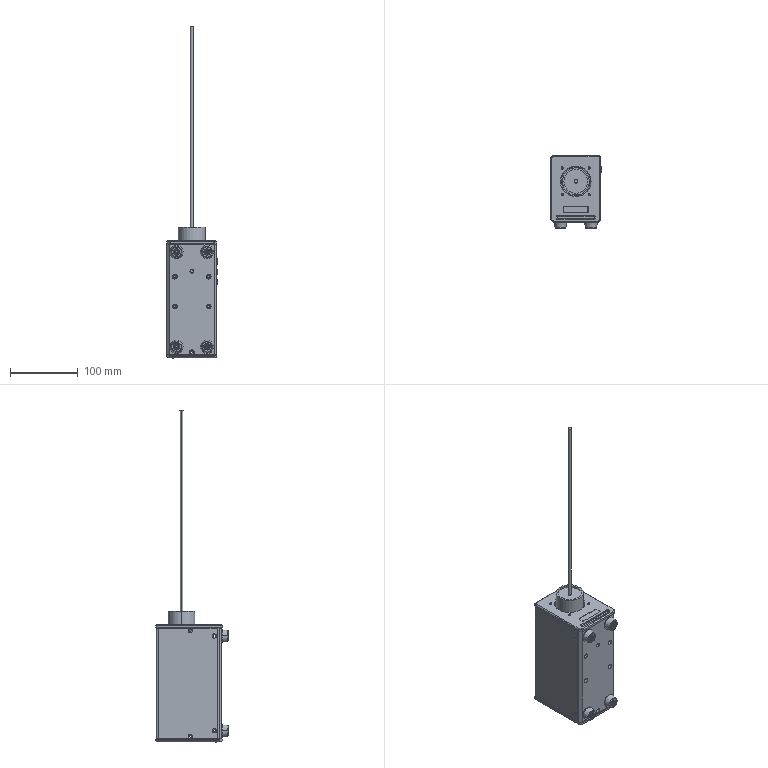Part | SolidWorks | 12 solids | 1026 faces | box 74.6 x 107 x 490 mm | volume 263242 mm3 | plane 511 | cylinder 199 | cone 177 | spline 139 | commonest cylinder face diameters 2 x46 3.4 x40 6.4 x14 10 x11 4 x10 8 x10